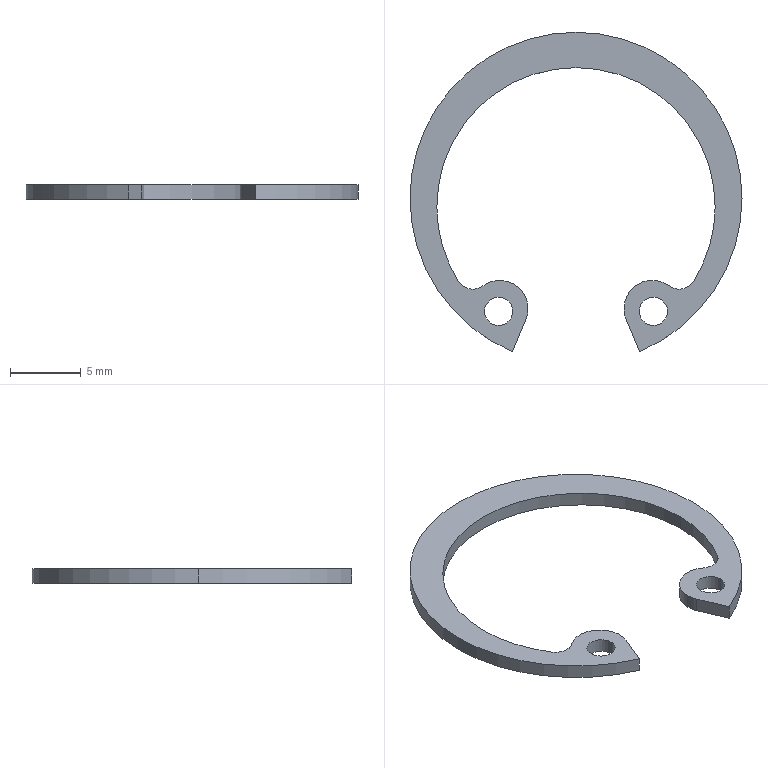Part | SolidWorks | features Extrusion 1 | 1 solid | 19 faces | box 23.5 x 22.606 x 1 mm | volume 131.088 mm3 | cylinder 15 | plane 4 | commonest cylinder face diameters 2 x4 4 x3 19.7 x3 23.5 x3 2.4 x2
STEP:
#1=CARTESIAN_POINT('',(4.48,-8.004,0.5));
#2=VERTEX_POINT('',#1);
#3=CARTESIAN_POINT('',(6.48,-8.004,0.5));
#4=VERTEX_POINT('',#3);
#5=CARTESIAN_POINT('',(5.48,-8.004,0.5));
#6=DIRECTION('',(0.,0.,1.));
#7=DIRECTION('',(-1.,0.,0.));
#8=AXIS2_PLACEMENT_3D('',#5,#6,#7);
#9=CIRCLE('',#8,1.);
#10=EDGE_CURVE('',#2,#4,#9,.T.);
#11=ORIENTED_EDGE('',*,*,#10,.T.);
#12=CARTESIAN_POINT('',(6.48,-8.004,-0.5));
#13=VERTEX_POINT('',#12);
#14=CARTESIAN_POINT('',(6.48,-8.004,0.5));
#15=DIRECTION('',(0.,0.,-1.));
#16=VECTOR('',#15,1000.);
#17=LINE('',#14,#16);
#18=EDGE_CURVE('',#4,#13,#17,.T.);
#19=ORIENTED_EDGE('',*,*,#18,.T.);
#20=CARTESIAN_POINT('',(4.48,-8.004,-0.5));
#21=VERTEX_POINT('',#20);
#22=CARTESIAN_POINT('',(5.48,-8.004,-0.5));
#23=DIRECTION('',(0.,0.,1.));
#24=DIRECTION('',(-1.,0.,0.));
#25=AXIS2_PLACEMENT_3D('',#22,#23,#24);
#26=CIRCLE('',#25,1.);
#27=EDGE_CURVE('',#21,#13,#26,.T.);
#28=ORIENTED_EDGE('',*,*,#27,.F.);
#29=CARTESIAN_POINT('',(4.48,-8.004,0.5));
#30=DIRECTION('',(0.,0.,-1.));
#31=VECTOR('',#30,1000.);
#32=LINE('',#29,#31);
#33=EDGE_CURVE('',#2,#21,#32,.T.);
#34=ORIENTED_EDGE('',*,*,#33,.F.);
#35=EDGE_LOOP('',(#11,#19,#28,#34));
#36=FACE_OUTER_BOUND('',#35,.T.);
#37=CARTESIAN_POINT('',(5.48,-8.004,0.5));
#38=DIRECTION('',(0.,0.,-1.));
#39=DIRECTION('',(-1.,0.,0.));
#40=AXIS2_PLACEMENT_3D('',#37,#38,#39);
#41=CYLINDRICAL_SURFACE('',#40,1.);
#42=ADVANCED_FACE('',(#36),#41,.F.);
#43=CARTESIAN_POINT('',(-6.48,-8.004,0.5));
#44=VERTEX_POINT('',#43);
#45=CARTESIAN_POINT('',(-4.48,-8.004,0.5));
#46=VERTEX_POINT('',#45);
#47=CARTESIAN_POINT('',(-5.48,-8.004,0.5));
#48=DIRECTION('',(0.,0.,1.));
#49=DIRECTION('',(1.,0.,0.));
#50=AXIS2_PLACEMENT_3D('',#47,#48,#49);
#51=CIRCLE('',#50,1.);
#52=EDGE_CURVE('',#44,#46,#51,.T.);
#53=ORIENTED_EDGE('',*,*,#52,.T.);
#54=CARTESIAN_POINT('',(-4.48,-8.004,-0.5));
#55=VERTEX_POINT('',#54);
#56=CARTESIAN_POINT('',(-4.48,-8.004,0.5));
#57=DIRECTION('',(0.,0.,-1.));
#58=VECTOR('',#57,1000.);
#59=LINE('',#56,#58);
#60=EDGE_CURVE('',#46,#55,#59,.T.);
#61=ORIENTED_EDGE('',*,*,#60,.T.);
#62=CARTESIAN_POINT('',(-6.48,-8.004,-0.5));
#63=VERTEX_POINT('',#62);
#64=CARTESIAN_POINT('',(-5.48,-8.004,-0.5));
#65=DIRECTION('',(0.,0.,1.));
#66=DIRECTION('',(1.,0.,0.));
#67=AXIS2_PLACEMENT_3D('',#64,#65,#66);
#68=CIRCLE('',#67,1.);
#69=EDGE_CURVE('',#63,#55,#68,.T.);
#70=ORIENTED_EDGE('',*,*,#69,.F.);
#71=CARTESIAN_POINT('',(-6.48,-8.004,0.5));
#72=DIRECTION('',(0.,0.,-1.));
#73=VECTOR('',#72,1000.);
#74=LINE('',#71,#73);
#75=EDGE_CURVE('',#44,#63,#74,.T.);
#76=ORIENTED_EDGE('',*,*,#75,.F.);
#77=EDGE_LOOP('',(#53,#61,#70,#76));
#78=FACE_OUTER_BOUND('',#77,.T.);
#79=CARTESIAN_POINT('',(-5.48,-8.004,0.5));
#80=DIRECTION('',(0.,0.,-1.));
#81=DIRECTION('',(-1.,0.,0.));
#82=AXIS2_PLACEMENT_3D('',#79,#80,#81);
#83=CYLINDRICAL_SURFACE('',#82,1.);
#84=ADVANCED_FACE('',(#78),#83,.F.);
#85=CARTESIAN_POINT('',(11.75,0.,0.5));
#86=VERTEX_POINT('',#85);
#87=CARTESIAN_POINT('',(-11.75,0.,0.5));
#88=VERTEX_POINT('',#87);
#89=CARTESIAN_POINT('',(0.,0.,0.5));
#90=DIRECTION('',(0.,0.,1.));
#91=DIRECTION('',(1.,0.,0.));
#92=AXIS2_PLACEMENT_3D('',#89,#90,#91);
#93=CIRCLE('',#92,11.75);
#94=EDGE_CURVE('',#86,#88,#93,.T.);
#95=ORIENTED_EDGE('',*,*,#94,.F.);
#96=CARTESIAN_POINT('',(11.75,0.,-0.5));
#97=VERTEX_POINT('',#96);
#98=CARTESIAN_POINT('',(11.75,0.,0.5));
#99=DIRECTION('',(0.,0.,-1.));
#100=VECTOR('',#99,1000.);
#101=LINE('',#98,#100);
#102=EDGE_CURVE('',#86,#97,#101,.T.);
#103=ORIENTED_EDGE('',*,*,#102,.T.);
#104=CARTESIAN_POINT('',(-11.75,0.,-0.5));
#105=VERTEX_POINT('',#104);
#106=CARTESIAN_POINT('',(0.,0.,-0.5));
#107=DIRECTION('',(0.,0.,1.));
#108=DIRECTION('',(1.,0.,0.));
#109=AXIS2_PLACEMENT_3D('',#106,#107,#108);
#110=CIRCLE('',#109,11.75);
#111=EDGE_CURVE('',#97,#105,#110,.T.);
#112=ORIENTED_EDGE('',*,*,#111,.T.);
#113=CARTESIAN_POINT('',(-11.75,0.,0.5));
#114=DIRECTION('',(0.,0.,-1.));
#115=VECTOR('',#114,1000.);
#116=LINE('',#113,#115);
#117=EDGE_CURVE('',#88,#105,#116,.T.);
#118=ORIENTED_EDGE('',*,*,#117,.F.);
#119=EDGE_LOOP('',(#95,#103,#112,#118));
#120=FACE_OUTER_BOUND('',#119,.T.);
#121=CARTESIAN_POINT('',(0.,0.,0.5));
#122=DIRECTION('',(0.,0.,-1.));
#123=DIRECTION('',(-1.,0.,0.));
#124=AXIS2_PLACEMENT_3D('',#121,#122,#123);
#125=CYLINDRICAL_SURFACE('',#124,11.75);
#126=ADVANCED_FACE('',(#120),#125,.T.);
#127=CARTESIAN_POINT('',(-4.497,-10.856,0.5));
#128=VERTEX_POINT('',#127);
#129=CARTESIAN_POINT('',(0.,0.,0.5));
#130=DIRECTION('',(0.,0.,1.));
#131=DIRECTION('',(1.,0.,0.));
#132=AXIS2_PLACEMENT_3D('',#129,#130,#131);
#133=CIRCLE('',#132,11.75);
#134=EDGE_CURVE('',#88,#128,#133,.T.);
#135=ORIENTED_EDGE('',*,*,#134,.F.);
#136=ORIENTED_EDGE('',*,*,#117,.T.);
#137=CARTESIAN_POINT('',(-4.497,-10.856,-0.5));
#138=VERTEX_POINT('',#137);
#139=CARTESIAN_POINT('',(0.,0.,-0.5));
#140=DIRECTION('',(0.,0.,1.));
#141=DIRECTION('',(1.,0.,0.));
#142=AXIS2_PLACEMENT_3D('',#139,#140,#141);
#143=CIRCLE('',#142,11.75);
#144=EDGE_CURVE('',#105,#138,#143,.T.);
#145=ORIENTED_EDGE('',*,*,#144,.T.);
#146=CARTESIAN_POINT('',(-4.497,-10.856,0.5));
#147=DIRECTION('',(0.,0.,-1.));
#148=VECTOR('',#147,1000.);
#149=LINE('',#146,#148);
#150=EDGE_CURVE('',#128,#138,#149,.T.);
#151=ORIENTED_EDGE('',*,*,#150,.F.);
#152=EDGE_LOOP('',(#135,#136,#145,#151));
#153=FACE_OUTER_BOUND('',#152,.T.);
#154=CARTESIAN_POINT('',(0.,0.,0.5));
#155=DIRECTION('',(0.,0.,-1.));
#156=DIRECTION('',(-1.,0.,0.));
#157=AXIS2_PLACEMENT_3D('',#154,#155,#156);
#158=CYLINDRICAL_SURFACE('',#157,11.75);
#159=ADVANCED_FACE('',(#153),#158,.T.);
#160=CARTESIAN_POINT('',(3.398,-7.805,0.5));
#161=VERTEX_POINT('',#160);
#162=CARTESIAN_POINT('',(3.55,-8.571,0.5));
#163=VERTEX_POINT('',#162);
#164=CARTESIAN_POINT('',(5.398,-7.805,0.5));
#165=DIRECTION('',(0.,0.,1.));
#166=DIRECTION('',(-1.,0.,0.));
#167=AXIS2_PLACEMENT_3D('',#164,#165,#166);
#168=CIRCLE('',#167,2.);
#169=EDGE_CURVE('',#161,#163,#168,.T.);
#170=ORIENTED_EDGE('',*,*,#169,.F.);
#171=CARTESIAN_POINT('',(3.398,-7.805,-0.5));
#172=VERTEX_POINT('',#171);
#173=CARTESIAN_POINT('',(3.398,-7.805,0.5));
#174=DIRECTION('',(0.,0.,-1.));
#175=VECTOR('',#174,1000.);
#176=LINE('',#173,#175);
#177=EDGE_CURVE('',#161,#172,#176,.T.);
#178=ORIENTED_EDGE('',*,*,#177,.T.);
#179=CARTESIAN_POINT('',(3.55,-8.571,-0.5));
#180=VERTEX_POINT('',#179);
#181=CARTESIAN_POINT('',(5.398,-7.805,-0.5));
#182=DIRECTION('',(0.,0.,1.));
#183=DIRECTION('',(-1.,0.,0.));
#184=AXIS2_PLACEMENT_3D('',#181,#182,#183);
#185=CIRCLE('',#184,2.);
#186=EDGE_CURVE('',#172,#180,#185,.T.);
#187=ORIENTED_EDGE('',*,*,#186,.T.);
#188=CARTESIAN_POINT('',(3.55,-8.571,0.5));
#189=DIRECTION('',(0.,0.,-1.));
#190=VECTOR('',#189,1000.);
#191=LINE('',#188,#190);
#192=EDGE_CURVE('',#163,#180,#191,.T.);
#193=ORIENTED_EDGE('',*,*,#192,.F.);
#194=EDGE_LOOP('',(#170,#178,#187,#193));
#195=FACE_OUTER_BOUND('',#194,.T.);
#196=CARTESIAN_POINT('',(5.398,-7.805,0.5));
#197=DIRECTION('',(0.,0.,-1.));
#198=DIRECTION('',(-1.,0.,0.));
#199=AXIS2_PLACEMENT_3D('',#196,#197,#198);
#200=CYLINDRICAL_SURFACE('',#199,2.);
#201=ADVANCED_FACE('',(#195),#200,.T.);
#202=CARTESIAN_POINT('',(9.85,-0.6,0.5));
#203=VERTEX_POINT('',#202);
#204=CARTESIAN_POINT('',(8.317,-5.878,0.5));
#205=VERTEX_POINT('',#204);
#206=CARTESIAN_POINT('',(0.,-0.6,0.5));
#207=DIRECTION('',(0.,0.,-1.));
#208=DIRECTION('',(1.,0.,0.));
#209=AXIS2_PLACEMENT_3D('',#206,#207,#208);
#210=CIRCLE('',#209,9.85);
#211=EDGE_CURVE('',#203,#205,#210,.T.);
#212=ORIENTED_EDGE('',*,*,#211,.F.);
#213=CARTESIAN_POINT('',(9.85,-0.6,-0.5));
#214=VERTEX_POINT('',#213);
#215=CARTESIAN_POINT('',(9.85,-0.6,0.5));
#216=DIRECTION('',(0.,0.,-1.));
#217=VECTOR('',#216,1000.);
#218=LINE('',#215,#217);
#219=EDGE_CURVE('',#203,#214,#218,.T.);
#220=ORIENTED_EDGE('',*,*,#219,.T.);
#221=CARTESIAN_POINT('',(8.317,-5.878,-0.5));
#222=VERTEX_POINT('',#221);
#223=CARTESIAN_POINT('',(0.,-0.6,-0.5));
#224=DIRECTION('',(0.,0.,-1.));
#225=DIRECTION('',(1.,0.,0.));
#226=AXIS2_PLACEMENT_3D('',#223,#224,#225);
#227=CIRCLE('',#226,9.85);
#228=EDGE_CURVE('',#214,#222,#227,.T.);
#229=ORIENTED_EDGE('',*,*,#228,.T.);
#230=CARTESIAN_POINT('',(8.317,-5.878,0.5));
#231=DIRECTION('',(0.,0.,-1.));
#232=VECTOR('',#231,1000.);
#233=LINE('',#230,#232);
#234=EDGE_CURVE('',#205,#222,#233,.T.);
#235=ORIENTED_EDGE('',*,*,#234,.F.);
#236=EDGE_LOOP('',(#212,#220,#229,#235));
#237=FACE_OUTER_BOUND('',#236,.T.);
#238=CARTESIAN_POINT('',(0.,-0.6,0.5));
#239=DIRECTION('',(0.,0.,-1.));
#240=DIRECTION('',(-1.,0.,0.));
#241=AXIS2_PLACEMENT_3D('',#238,#239,#240);
#242=CYLINDRICAL_SURFACE('',#241,9.85);
#243=ADVANCED_FACE('',(#237),#242,.F.);
#244=ORIENTED_EDGE('',*,*,#219,.F.);
#245=CARTESIAN_POINT('',(-9.85,-0.6,0.5));
#246=VERTEX_POINT('',#245);
#247=CARTESIAN_POINT('',(0.,-0.6,0.5));
#248=DIRECTION('',(0.,0.,-1.));
#249=DIRECTION('',(1.,0.,0.));
#250=AXIS2_PLACEMENT_3D('',#247,#248,#249);
#251=CIRCLE('',#250,9.85);
#252=EDGE_CURVE('',#246,#203,#251,.T.);
#253=ORIENTED_EDGE('',*,*,#252,.F.);
#254=CARTESIAN_POINT('',(-9.85,-0.6,-0.5));
#255=VERTEX_POINT('',#254);
#256=CARTESIAN_POINT('',(-9.85,-0.6,0.5));
#257=DIRECTION('',(0.,0.,-1.));
#258=VECTOR('',#257,1000.);
#259=LINE('',#256,#258);
#260=EDGE_CURVE('',#246,#255,#259,.T.);
#261=ORIENTED_EDGE('',*,*,#260,.T.);
#262=CARTESIAN_POINT('',(0.,-0.6,-0.5));
#263=DIRECTION('',(0.,0.,-1.));
#264=DIRECTION('',(1.,0.,0.));
#265=AXIS2_PLACEMENT_3D('',#262,#263,#264);
#266=CIRCLE('',#265,9.85);
#267=EDGE_CURVE('',#255,#214,#266,.T.);
#268=ORIENTED_EDGE('',*,*,#267,.T.);
#269=EDGE_LOOP('',(#244,#253,#261,#268));
#270=FACE_OUTER_BOUND('',#269,.T.);
#271=CARTESIAN_POINT('',(0.,-0.6,0.5));
#272=DIRECTION('',(0.,0.,-1.));
#273=DIRECTION('',(-1.,0.,0.));
#274=AXIS2_PLACEMENT_3D('',#271,#272,#273);
#275=CYLINDRICAL_SURFACE('',#274,9.85);
#276=ADVANCED_FACE('',(#270),#275,.F.);
#277=ORIENTED_EDGE('',*,*,#52,.F.);
#278=CARTESIAN_POINT('',(-5.48,-8.004,0.5));
#279=DIRECTION('',(0.,0.,1.));
#280=DIRECTION('',(1.,0.,0.));
#281=AXIS2_PLACEMENT_3D('',#278,#279,#280);
#282=CIRCLE('',#281,1.);
#283=EDGE_CURVE('',#46,#44,#282,.T.);
#284=ORIENTED_EDGE('',*,*,#283,.F.);
#285=EDGE_LOOP('',(#277,#284));
#286=FACE_BOUND('',#285,.T.);
#287=CARTESIAN_POINT('',(-3.55,-8.571,0.5));
#288=VERTEX_POINT('',#287);
#289=CARTESIAN_POINT('',(-6.589,-6.199,0.5));
#290=VERTEX_POINT('',#289);
#291=CARTESIAN_POINT('',(-5.398,-7.805,0.5));
#292=DIRECTION('',(0.,0.,1.));
#293=DIRECTION('',(1.,0.,0.));
#294=AXIS2_PLACEMENT_3D('',#291,#292,#293);
#295=CIRCLE('',#294,2.);
#296=EDGE_CURVE('',#288,#290,#295,.T.);
#297=ORIENTED_EDGE('',*,*,#296,.T.);
#298=CARTESIAN_POINT('',(-8.317,-5.878,0.5));
#299=VERTEX_POINT('',#298);
#300=CARTESIAN_POINT('',(-7.304,-5.235,0.5));
#301=DIRECTION('',(0.,0.,-1.));
#302=DIRECTION('',(-1.,0.,0.));
#303=AXIS2_PLACEMENT_3D('',#300,#301,#302);
#304=CIRCLE('',#303,1.2);
#305=EDGE_CURVE('',#290,#299,#304,.T.);
#306=ORIENTED_EDGE('',*,*,#305,.T.);
#307=CARTESIAN_POINT('',(0.,-0.6,0.5));
#308=DIRECTION('',(0.,0.,-1.));
#309=DIRECTION('',(1.,0.,0.));
#310=AXIS2_PLACEMENT_3D('',#307,#308,#309);
#311=CIRCLE('',#310,9.85);
#312=EDGE_CURVE('',#299,#246,#311,.T.);
#313=ORIENTED_EDGE('',*,*,#312,.T.);
#314=ORIENTED_EDGE('',*,*,#252,.T.);
#315=ORIENTED_EDGE('',*,*,#211,.T.);
#316=CARTESIAN_POINT('',(6.589,-6.199,0.5));
#317=VERTEX_POINT('',#316);
#318=CARTESIAN_POINT('',(7.304,-5.235,0.5));
#319=DIRECTION('',(0.,0.,-1.));
#320=DIRECTION('',(1.,0.,0.));
#321=AXIS2_PLACEMENT_3D('',#318,#319,#320);
#322=CIRCLE('',#321,1.2);
#323=EDGE_CURVE('',#205,#317,#322,.T.);
#324=ORIENTED_EDGE('',*,*,#323,.T.);
#325=CARTESIAN_POINT('',(5.398,-7.805,0.5));
#326=DIRECTION('',(0.,0.,1.));
#327=DIRECTION('',(-1.,0.,0.));
#328=AXIS2_PLACEMENT_3D('',#325,#326,#327);
#329=CIRCLE('',#328,2.);
#330=EDGE_CURVE('',#317,#161,#329,.T.);
#331=ORIENTED_EDGE('',*,*,#330,.T.);
#332=ORIENTED_EDGE('',*,*,#169,.T.);
#333=CARTESIAN_POINT('',(4.497,-10.856,0.5));
#334=VERTEX_POINT('',#333);
#335=CARTESIAN_POINT('',(3.55,-8.571,0.5));
#336=DIRECTION('',(0.3827,-0.9239,0.));
#337=VECTOR('',#336,1000.);
#338=LINE('',#335,#337);
#339=EDGE_CURVE('',#163,#334,#338,.T.);
#340=ORIENTED_EDGE('',*,*,#339,.T.);
#341=CARTESIAN_POINT('',(0.,0.,0.5));
#342=DIRECTION('',(0.,0.,1.));
#343=DIRECTION('',(1.,0.,0.));
#344=AXIS2_PLACEMENT_3D('',#341,#342,#343);
#345=CIRCLE('',#344,11.75);
#346=EDGE_CURVE('',#334,#86,#345,.T.);
#347=ORIENTED_EDGE('',*,*,#346,.T.);
#348=ORIENTED_EDGE('',*,*,#94,.T.);
#349=ORIENTED_EDGE('',*,*,#134,.T.);
#350=CARTESIAN_POINT('',(-3.55,-8.571,0.5));
#351=DIRECTION('',(0.3827,0.9239,0.));
#352=VECTOR('',#351,1000.);
#353=LINE('',#350,#352);
#354=EDGE_CURVE('',#128,#288,#353,.T.);
#355=ORIENTED_EDGE('',*,*,#354,.T.);
#356=EDGE_LOOP('',(#297,#306,#313,#314,#315,#324,#331,#332,#340,#347,#348,#349,#355));
#357=FACE_OUTER_BOUND('',#356,.T.);
#358=ORIENTED_EDGE('',*,*,#10,.F.);
#359=CARTESIAN_POINT('',(5.48,-8.004,0.5));
#360=DIRECTION('',(0.,0.,1.));
#361=DIRECTION('',(-1.,0.,0.));
#362=AXIS2_PLACEMENT_3D('',#359,#360,#361);
#363=CIRCLE('',#362,1.);
#364=EDGE_CURVE('',#4,#2,#363,.T.);
#365=ORIENTED_EDGE('',*,*,#364,.F.);
#366=EDGE_LOOP('',(#358,#365));
#367=FACE_BOUND('',#366,.T.);
#368=CARTESIAN_POINT('',(-5.398,-7.805,0.5));
#369=DIRECTION('',(0.,0.,1.));
#370=DIRECTION('',(1.,0.,0.));
#371=AXIS2_PLACEMENT_3D('',#368,#369,#370);
#372=PLANE('',#371);
#373=ADVANCED_FACE('',(#286,#357,#367),#372,.T.);
#374=CARTESIAN_POINT('',(-3.55,-8.571,-0.5));
#375=VERTEX_POINT('',#374);
#376=CARTESIAN_POINT('',(-3.55,-8.571,0.5));
#377=DIRECTION('',(0.,0.,-1.));
#378=VECTOR('',#377,1000.);
#379=LINE('',#376,#378);
#380=EDGE_CURVE('',#288,#375,#379,.T.);
#381=ORIENTED_EDGE('',*,*,#380,.T.);
#382=CARTESIAN_POINT('',(-6.589,-6.199,-0.5));
#383=VERTEX_POINT('',#382);
#384=CARTESIAN_POINT('',(-5.398,-7.805,-0.5));
#385=DIRECTION('',(0.,0.,1.));
#386=DIRECTION('',(1.,0.,0.));
#387=AXIS2_PLACEMENT_3D('',#384,#385,#386);
#388=CIRCLE('',#387,2.);
#389=EDGE_CURVE('',#375,#383,#388,.T.);
#390=ORIENTED_EDGE('',*,*,#389,.T.);
#391=CARTESIAN_POINT('',(-6.589,-6.199,0.5));
#392=DIRECTION('',(0.,0.,-1.));
#393=VECTOR('',#392,1000.);
#394=LINE('',#391,#393);
#395=EDGE_CURVE('',#290,#383,#394,.T.);
#396=ORIENTED_EDGE('',*,*,#395,.F.);
#397=ORIENTED_EDGE('',*,*,#296,.F.);
#398=EDGE_LOOP('',(#381,#390,#396,#397));
#399=FACE_OUTER_BOUND('',#398,.T.);
#400=CARTESIAN_POINT('',(-5.398,-7.805,0.5));
#401=DIRECTION('',(0.,0.,-1.));
#402=DIRECTION('',(-1.,0.,0.));
#403=AXIS2_PLACEMENT_3D('',#400,#401,#402);
#404=CYLINDRICAL_SURFACE('',#403,2.);
#405=ADVANCED_FACE('',(#399),#404,.T.);
#406=ORIENTED_EDGE('',*,*,#395,.T.);
#407=CARTESIAN_POINT('',(-8.317,-5.878,-0.5));
#408=VERTEX_POINT('',#407);
#409=CARTESIAN_POINT('',(-7.304,-5.235,-0.5));
#410=DIRECTION('',(0.,0.,-1.));
#411=DIRECTION('',(-1.,0.,0.));
#412=AXIS2_PLACEMENT_3D('',#409,#410,#411);
#413=CIRCLE('',#412,1.2);
#414=EDGE_CURVE('',#383,#408,#413,.T.);
#415=ORIENTED_EDGE('',*,*,#414,.T.);
#416=CARTESIAN_POINT('',(-8.317,-5.878,0.5));
#417=DIRECTION('',(0.,0.,-1.));
#418=VECTOR('',#417,1000.);
#419=LINE('',#416,#418);
#420=EDGE_CURVE('',#299,#408,#419,.T.);
#421=ORIENTED_EDGE('',*,*,#420,.F.);
#422=ORIENTED_EDGE('',*,*,#305,.F.);
#423=EDGE_LOOP('',(#406,#415,#421,#422));
#424=FACE_OUTER_BOUND('',#423,.T.);
#425=CARTESIAN_POINT('',(-7.304,-5.235,0.5));
#426=DIRECTION('',(0.,0.,-1.));
#427=DIRECTION('',(-1.,0.,0.));
#428=AXIS2_PLACEMENT_3D('',#425,#426,#427);
#429=CYLINDRICAL_SURFACE('',#428,1.2);
#430=ADVANCED_FACE('',(#424),#429,.F.);
#431=ORIENTED_EDGE('',*,*,#260,.F.);
#432=ORIENTED_EDGE('',*,*,#312,.F.);
#433=ORIENTED_EDGE('',*,*,#420,.T.);
#434=CARTESIAN_POINT('',(0.,-0.6,-0.5));
#435=DIRECTION('',(0.,0.,-1.));
#436=DIRECTION('',(1.,0.,0.));
#437=AXIS2_PLACEMENT_3D('',#434,#435,#436);
#438=CIRCLE('',#437,9.85);
#439=EDGE_CURVE('',#408,#255,#438,.T.);
#440=ORIENTED_EDGE('',*,*,#439,.T.);
#441=EDGE_LOOP('',(#431,#432,#433,#440));
#442=FACE_OUTER_BOUND('',#441,.T.);
#443=CARTESIAN_POINT('',(0.,-0.6,0.5));
#444=DIRECTION('',(0.,0.,-1.));
#445=DIRECTION('',(-1.,0.,0.));
#446=AXIS2_PLACEMENT_3D('',#443,#444,#445);
#447=CYLINDRICAL_SURFACE('',#446,9.85);
#448=ADVANCED_FACE('',(#442),#447,.F.);
#449=ORIENTED_EDGE('',*,*,#234,.T.);
#450=CARTESIAN_POINT('',(6.589,-6.199,-0.5));
#451=VERTEX_POINT('',#450);
#452=CARTESIAN_POINT('',(7.304,-5.235,-0.5));
#453=DIRECTION('',(0.,0.,-1.));
#454=DIRECTION('',(1.,0.,0.));
#455=AXIS2_PLACEMENT_3D('',#452,#453,#454);
#456=CIRCLE('',#455,1.2);
#457=EDGE_CURVE('',#222,#451,#456,.T.);
#458=ORIENTED_EDGE('',*,*,#457,.T.);
#459=CARTESIAN_POINT('',(6.589,-6.199,0.5));
#460=DIRECTION('',(0.,0.,-1.));
#461=VECTOR('',#460,1000.);
#462=LINE('',#459,#461);
#463=EDGE_CURVE('',#317,#451,#462,.T.);
#464=ORIENTED_EDGE('',*,*,#463,.F.);
#465=ORIENTED_EDGE('',*,*,#323,.F.);
#466=EDGE_LOOP('',(#449,#458,#464,#465));
#467=FACE_OUTER_BOUND('',#466,.T.);
#468=CARTESIAN_POINT('',(7.304,-5.235,0.5));
#469=DIRECTION('',(0.,0.,-1.));
#470=DIRECTION('',(-1.,0.,0.));
#471=AXIS2_PLACEMENT_3D('',#468,#469,#470);
#472=CYLINDRICAL_SURFACE('',#471,1.2);
#473=ADVANCED_FACE('',(#467),#472,.F.);
#474=ORIENTED_EDGE('',*,*,#177,.F.);
#475=ORIENTED_EDGE('',*,*,#330,.F.);
#476=ORIENTED_EDGE('',*,*,#463,.T.);
#477=CARTESIAN_POINT('',(5.398,-7.805,-0.5));
#478=DIRECTION('',(0.,0.,1.));
#479=DIRECTION('',(-1.,0.,0.));
#480=AXIS2_PLACEMENT_3D('',#477,#478,#479);
#481=CIRCLE('',#480,2.);
#482=EDGE_CURVE('',#451,#172,#481,.T.);
#483=ORIENTED_EDGE('',*,*,#482,.T.);
#484=EDGE_LOOP('',(#474,#475,#476,#483));
#485=FACE_OUTER_BOUND('',#484,.T.);
#486=CARTESIAN_POINT('',(5.398,-7.805,0.5));
#487=DIRECTION('',(0.,0.,-1.));
#488=DIRECTION('',(-1.,0.,0.));
#489=AXIS2_PLACEMENT_3D('',#486,#487,#488);
#490=CYLINDRICAL_SURFACE('',#489,2.);
#491=ADVANCED_FACE('',(#485),#490,.T.);
#492=ORIENTED_EDGE('',*,*,#192,.T.);
#493=CARTESIAN_POINT('',(4.497,-10.856,-0.5));
#494=VERTEX_POINT('',#493);
#495=CARTESIAN_POINT('',(3.55,-8.571,-0.5));
#496=DIRECTION('',(0.3827,-0.9239,0.));
#497=VECTOR('',#496,1000.);
#498=LINE('',#495,#497);
#499=EDGE_CURVE('',#180,#494,#498,.T.);
#500=ORIENTED_EDGE('',*,*,#499,.T.);
#501=CARTESIAN_POINT('',(4.497,-10.856,0.5));
#502=DIRECTION('',(0.,0.,-1.));
#503=VECTOR('',#502,1000.);
#504=LINE('',#501,#503);
#505=EDGE_CURVE('',#334,#494,#504,.T.);
#506=ORIENTED_EDGE('',*,*,#505,.F.);
#507=ORIENTED_EDGE('',*,*,#339,.F.);
#508=EDGE_LOOP('',(#492,#500,#506,#507));
#509=FACE_OUTER_BOUND('',#508,.T.);
#510=CARTESIAN_POINT('',(3.55,-8.571,0.5));
#511=DIRECTION('',(0.9239,0.3827,0.));
#512=DIRECTION('',(-0.3827,0.9239,0.));
#513=AXIS2_PLACEMENT_3D('',#510,#511,#512);
#514=PLANE('',#513);
#515=ADVANCED_FACE('',(#509),#514,.F.);
#516=ORIENTED_EDGE('',*,*,#102,.F.);
#517=ORIENTED_EDGE('',*,*,#346,.F.);
#518=ORIENTED_EDGE('',*,*,#505,.T.);
#519=CARTESIAN_POINT('',(0.,0.,-0.5));
#520=DIRECTION('',(0.,0.,1.));
#521=DIRECTION('',(1.,0.,0.));
#522=AXIS2_PLACEMENT_3D('',#519,#520,#521);
#523=CIRCLE('',#522,11.75);
#524=EDGE_CURVE('',#494,#97,#523,.T.);
#525=ORIENTED_EDGE('',*,*,#524,.T.);
#526=EDGE_LOOP('',(#516,#517,#518,#525));
#527=FACE_OUTER_BOUND('',#526,.T.);
#528=CARTESIAN_POINT('',(0.,0.,0.5));
#529=DIRECTION('',(0.,0.,-1.));
#530=DIRECTION('',(-1.,0.,0.));
#531=AXIS2_PLACEMENT_3D('',#528,#529,#530);
#532=CYLINDRICAL_SURFACE('',#531,11.75);
#533=ADVANCED_FACE('',(#527),#532,.T.);
#534=ORIENTED_EDGE('',*,*,#150,.T.);
#535=CARTESIAN_POINT('',(-3.55,-8.571,-0.5));
#536=DIRECTION('',(0.3827,0.9239,0.));
#537=VECTOR('',#536,1000.);
#538=LINE('',#535,#537);
#539=EDGE_CURVE('',#138,#375,#538,.T.);
#540=ORIENTED_EDGE('',*,*,#539,.T.);
#541=ORIENTED_EDGE('',*,*,#380,.F.);
#542=ORIENTED_EDGE('',*,*,#354,.F.);
#543=EDGE_LOOP('',(#534,#540,#541,#542));
#544=FACE_OUTER_BOUND('',#543,.T.);
#545=CARTESIAN_POINT('',(-3.55,-8.571,0.5));
#546=DIRECTION('',(-0.9239,0.3827,0.));
#547=DIRECTION('',(-0.3827,-0.9239,0.));
#548=AXIS2_PLACEMENT_3D('',#545,#546,#547);
#549=PLANE('',#548);
#550=ADVANCED_FACE('',(#544),#549,.F.);
#551=ORIENTED_EDGE('',*,*,#60,.F.);
#552=ORIENTED_EDGE('',*,*,#283,.T.);
#553=ORIENTED_EDGE('',*,*,#75,.T.);
#554=CARTESIAN_POINT('',(-5.48,-8.004,-0.5));
#555=DIRECTION('',(0.,0.,1.));
#556=DIRECTION('',(1.,0.,0.));
#557=AXIS2_PLACEMENT_3D('',#554,#555,#556);
#558=CIRCLE('',#557,1.);
#559=EDGE_CURVE('',#55,#63,#558,.T.);
#560=ORIENTED_EDGE('',*,*,#559,.F.);
#561=EDGE_LOOP('',(#551,#552,#553,#560));
#562=FACE_OUTER_BOUND('',#561,.T.);
#563=CARTESIAN_POINT('',(-5.48,-8.004,0.5));
#564=DIRECTION('',(0.,0.,-1.));
#565=DIRECTION('',(-1.,0.,0.));
#566=AXIS2_PLACEMENT_3D('',#563,#564,#565);
#567=CYLINDRICAL_SURFACE('',#566,1.);
#568=ADVANCED_FACE('',(#562),#567,.F.);
#569=ORIENTED_EDGE('',*,*,#18,.F.);
#570=ORIENTED_EDGE('',*,*,#364,.T.);
#571=ORIENTED_EDGE('',*,*,#33,.T.);
#572=CARTESIAN_POINT('',(5.48,-8.004,-0.5));
#573=DIRECTION('',(0.,0.,1.));
#574=DIRECTION('',(-1.,0.,0.));
#575=AXIS2_PLACEMENT_3D('',#572,#573,#574);
#576=CIRCLE('',#575,1.);
#577=EDGE_CURVE('',#13,#21,#576,.T.);
#578=ORIENTED_EDGE('',*,*,#577,.F.);
#579=EDGE_LOOP('',(#569,#570,#571,#578));
#580=FACE_OUTER_BOUND('',#579,.T.);
#581=CARTESIAN_POINT('',(5.48,-8.004,0.5));
#582=DIRECTION('',(0.,0.,-1.));
#583=DIRECTION('',(-1.,0.,0.));
#584=AXIS2_PLACEMENT_3D('',#581,#582,#583);
#585=CYLINDRICAL_SURFACE('',#584,1.);
#586=ADVANCED_FACE('',(#580),#585,.F.);
#587=ORIENTED_EDGE('',*,*,#27,.T.);
#588=ORIENTED_EDGE('',*,*,#577,.T.);
#589=EDGE_LOOP('',(#587,#588));
#590=FACE_BOUND('',#589,.T.);
#591=ORIENTED_EDGE('',*,*,#69,.T.);
#592=ORIENTED_EDGE('',*,*,#559,.T.);
#593=EDGE_LOOP('',(#591,#592));
#594=FACE_BOUND('',#593,.T.);
#595=ORIENTED_EDGE('',*,*,#389,.F.);
#596=ORIENTED_EDGE('',*,*,#539,.F.);
#597=ORIENTED_EDGE('',*,*,#144,.F.);
#598=ORIENTED_EDGE('',*,*,#111,.F.);
#599=ORIENTED_EDGE('',*,*,#524,.F.);
#600=ORIENTED_EDGE('',*,*,#499,.F.);
#601=ORIENTED_EDGE('',*,*,#186,.F.);
#602=ORIENTED_EDGE('',*,*,#482,.F.);
#603=ORIENTED_EDGE('',*,*,#457,.F.);
#604=ORIENTED_EDGE('',*,*,#228,.F.);
#605=ORIENTED_EDGE('',*,*,#267,.F.);
#606=ORIENTED_EDGE('',*,*,#439,.F.);
#607=ORIENTED_EDGE('',*,*,#414,.F.);
#608=EDGE_LOOP('',(#595,#596,#597,#598,#599,#600,#601,#602,#603,#604,#605,#606,#607));
#609=FACE_OUTER_BOUND('',#608,.T.);
#610=CARTESIAN_POINT('',(-5.398,-7.805,-0.5));
#611=DIRECTION('',(0.,0.,1.));
#612=DIRECTION('',(1.,0.,0.));
#613=AXIS2_PLACEMENT_3D('',#610,#611,#612);
#614=PLANE('',#613);
#615=ADVANCED_FACE('',(#590,#594,#609),#614,.F.);
#616=CLOSED_SHELL('',(#42,#84,#126,#159,#201,#243,#276,#373,#405,#430,#448,#473,#491,#515,#533,#550,#568,#586,#615));
#617=MANIFOLD_SOLID_BREP('',#616);
#618=CARTESIAN_POINT('',(0.,0.,0.));
#619=DIRECTION('',(0.,0.,1.));
#620=DIRECTION('',(1.,0.,0.));
#621=AXIS2_PLACEMENT_3D('',#618,#619,#620);
#622=(LENGTH_UNIT()NAMED_UNIT(*)SI_UNIT(.MILLI.,.METRE.));
#623=UNCERTAINTY_MEASURE_WITH_UNIT(LENGTH_MEASURE(0.00001),#622,'','');
#624=(NAMED_UNIT(*)PLANE_ANGLE_UNIT()SI_UNIT($,.RADIAN.));
#625=(NAMED_UNIT(*)SI_UNIT($,.STERADIAN.)SOLID_ANGLE_UNIT());
#626=(GEOMETRIC_REPRESENTATION_CONTEXT(3)GLOBAL_UNCERTAINTY_ASSIGNED_CONTEXT((#623))GLOBAL_UNIT_ASSIGNED_CONTEXT((#622,#624,#625))REPRESENTATION_CONTEXT('',''));
#627=ADVANCED_BREP_SHAPE_REPRESENTATION('',(#617,#621),#626);